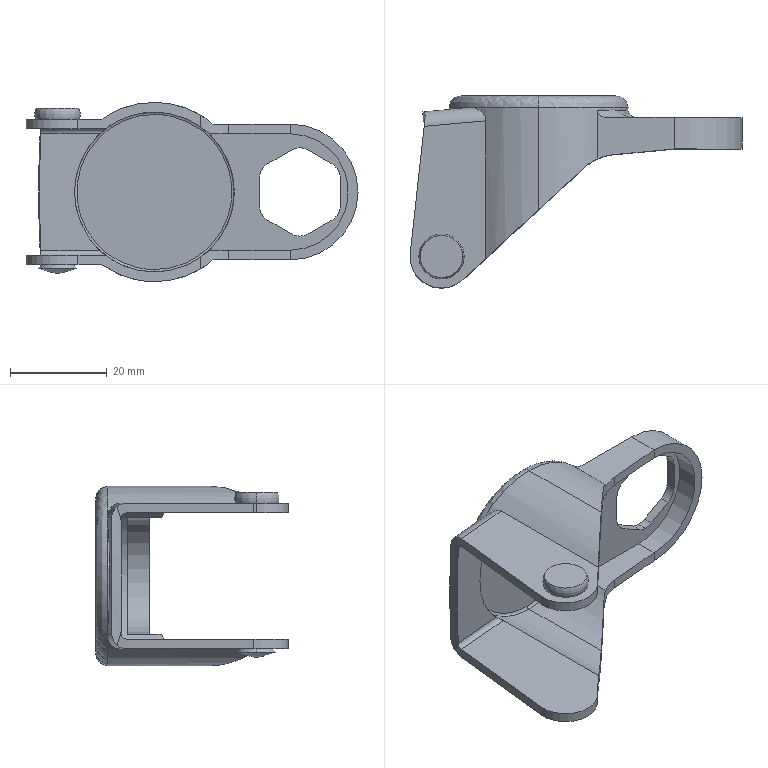Part | STEP file | _CMAZ40-N_b | 1 solid | 63 faces | box 68.5 x 39.7 x 37 mm | volume 8517 mm3 | plane 28 | cylinder 25 | spline 6 | cone 2 | torus 2 | commonest cylinder face diameters 7 x7 37 x4 13 x3 2 x2 6 x2 20 x2